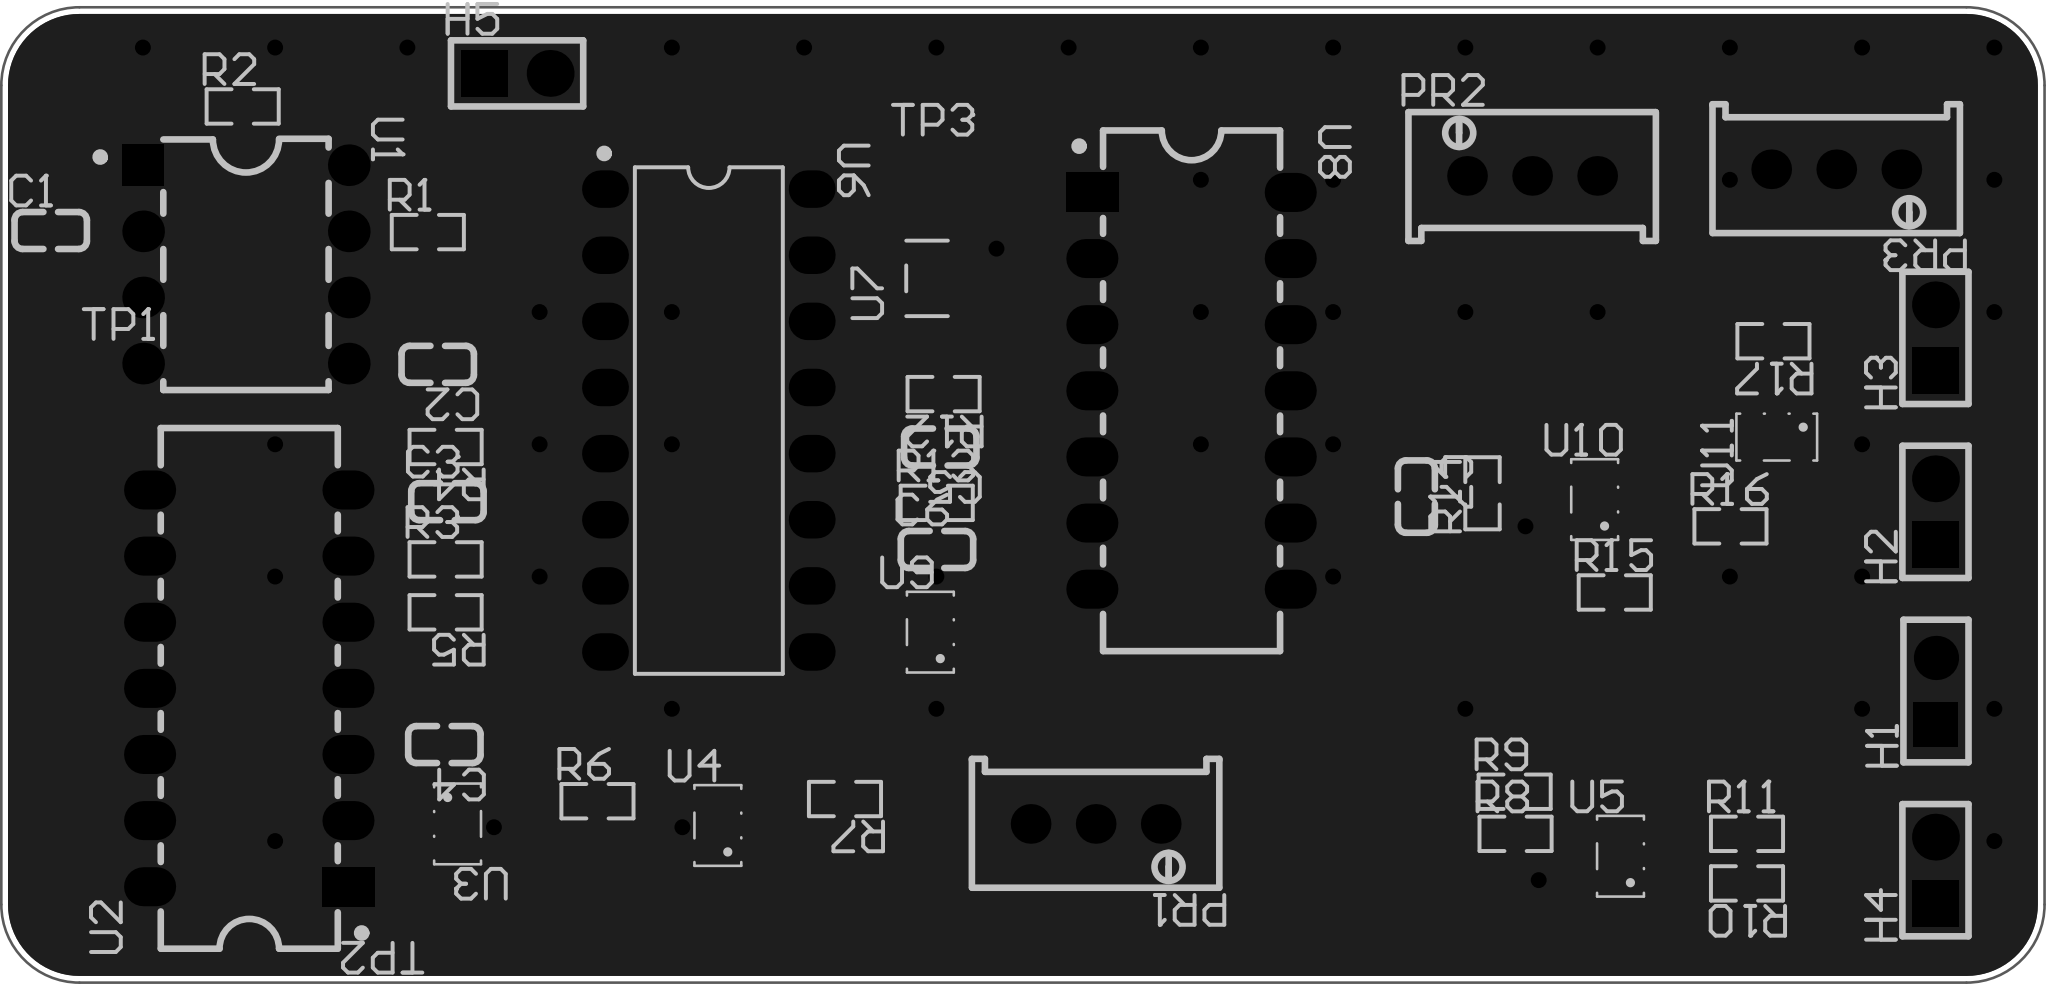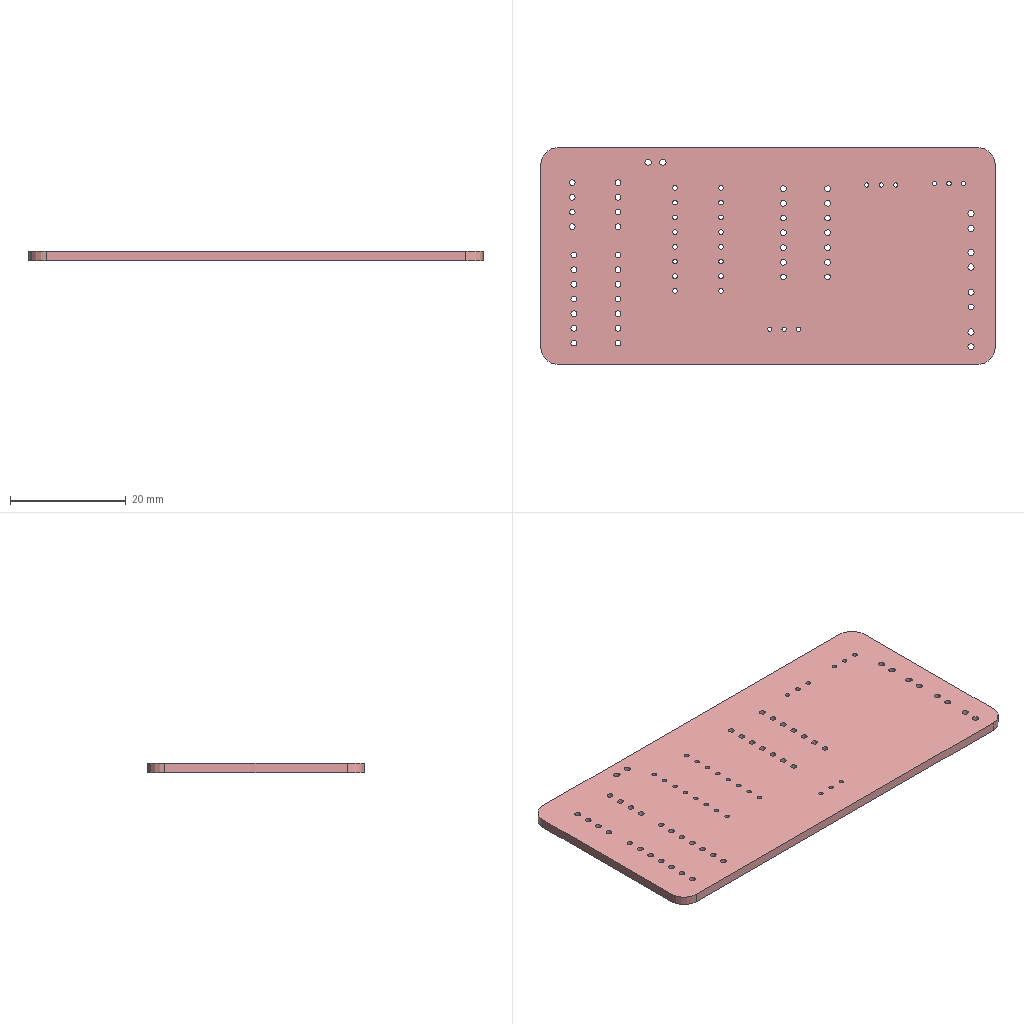Circuit board layout | Altium Designer | box 78.5 x 37.5 x 1.6 mm
Layer stack:
# Altium Designer layer stack of  (unit mm; dielectric type: 0 none, 1 core, 2 prepreg, 3 surface material)
index,name,kind,layer,copper_thickness_mm,dielectric_type,dielectric_thickness_mm,dielectric_material,dielectric_constant
0,Top Paste Mask Layer,other,,,,,,
1,Top Silkscreen Layer,other,,,,,,
2,Top Solder Mask Layer,dielectric,,,3,0.01,,3.3
3,Top Layer,copper,Top Layer,0.035,,,,
4,Dielectric1,dielectric,,,3,1.51,FR4,4.5
5,Bottom Layer,copper,Bottom Layer,0.035,,,,
6,Bottom Solder Mask Layer,dielectric,,,3,0.01,,3.3
7,Bottom Silkscreen Layer,other,,,,,,
8,Bottom Paste Mask Layer,other,,,,,,
# drill layer pairs: low layer,high layer
drill_pair,Top Layer,Bottom Layer
Part placement:
Designator,Comment,Layer,Footprint,Center-X(mm),Center-Y(mm),Rotation
C1,5nF,TopLayer,C0603,79.876,108.011,0
C2,0.22uF,TopLayer,C0603,94.742,102.87,180
C3,5.1nF,TopLayer,C0603,95.114,97.596,0
C4,1nF,TopLayer,C0603,94.996,88.265,180
C5,3300pF,TopLayer,C0603,114.046,99.695,180
C6,3300pF,TopLayer,C0603,113.919,95.758,0
C7,1nF,TopLayer,C0603,132.334,97.79,270
H1,,TopLayer,HDR-TH_2P-P2.54-V-F,152.293,90.321,90
H2,,TopLayer,HDR-TH_2P-P2.54-V-M-1,152.273,97.204,90
H3,,TopLayer,HDR-TH_2P-P2.54-V-M-1,152.273,103.886,90
H4,,TopLayer,HDR-TH_2P-P2.54-V-M-1,152.273,83.439,90
PR1,10kΩ,TopLayer,R_3296,120.015,85.217,180
PR2,10kΩ,TopLayer,R_3296,136.779,110.109,0
PR3,10kΩ,TopLayer,R_3296,148.463,110.363,180
R1,1.2K,TopLayer,R0603,94.361,107.95,0
R2,1.8K,TopLayer,R0603,87.249,112.776,0
R3,2K,TopLayer,R0603,95.044,95.377,0
R4,2K,TopLayer,R0603,95.044,99.695,180
R5,2.7K,TopLayer,R0603,95.044,93.345,180
R6,2K,TopLayer,R0603,100.877,86.089,0
R7,2K,TopLayer,R0603,110.385,86.173,180
R8,10K,TopLayer,R0603,136.144,84.836,0
R9,10K,TopLayer,R0603,136.109,86.453,0
R10,10K,TopLayer,R0603,145.034,82.931,180
R11,10K,TopLayer,R0603,145.034,84.836,0
R12,5.1K,TopLayer,R0603,114.173,101.727,180
R13,5.1K,TopLayer,R0603,113.909,97.549,0
R14,10K,TopLayer,R0603,134.874,97.917,90
R15,10K,TopLayer,R0603,139.954,94.107,0
R16,2K,TopLayer,R0603,144.399,96.647,0
R17,2K,TopLayer,R0603,146.05,103.759,180
TP1,,TopLayer,Test-Point-0.5mm,81.394,103.471,0
TP2,,TopLayer,Test-Point-0.5mm,93.901,81.026,180
TP3,,TopLayer,Test-Point-0.5mm,112.478,111.318,0
U1,NE555,TopLayer,PDIP-8_L9.6-W6.4-P2.54-LS7.9-BL-1,87.375,106.709,270
U2,DM7474N,TopLayer,PDIP-14_L19.5-W6.7-P2.54-LS7.9-BL,87.503,90.424,90
U3,OPAMP_3T_VIRTUAL,TopLayer,SOT-23-5_L3.0-W1.7-P0.95-LS2.8-BR,95.504,85.217,180
U4,OPAMP_3T_VIRTUAL,TopLayer,SOT-23-5_L3.0-W1.7-P0.95-LS2.8-BR,105.502,85.157,0
U5,OPAMP_3T_VIRTUAL,TopLayer,SOT-23-5_L3.0-W1.7-P0.95-LS2.8-BR,140.175,83.976,0
U6,74LS161N,TopLayer,PDIP-16_L19.3-W6.4-P2.54-LS7.94-BL,105.156,100.711,270
U7,HSN74LVC1G04DBVR,TopLayer,SOT-23-5_L2.9-W1.6-P0.95-LS2.9-BL,113.538,106.172,90
U8,DM7474N,TopLayer,PDIP-14_L19.5-W6.7-P2.54-LS7.9-BL,123.698,101.854,270
U9,OPAMP_3T_VIRTUAL,TopLayer,SOT-23-5_L3.0-W1.7-P0.95-LS2.8-BR,113.665,92.583,0
U10,OPAMP_3T_VIRTUAL,TopLayer,SOT-23-5_L3.0-W1.7-P0.95-LS2.8-BR,139.182,97.676,0
U11,OPAMP_3T_VIRTUAL,TopLayer,SOT-23-5_L3.0-W1.7-P0.95-LS2.8-BR,146.177,100.076,90
H5,,TopLayer,HDR-TH_2P-P2.54-V-M-1,97.79,114.046,0
Pad and via stacks:
# Altium Designer via and pad stacks of  (unit mm). Each distinct definition once, with the count of objects using it.
# via: kind,start_layer,end_layer,hole_mm,diameter_mm,mode(0 simple;1 top-mid-bottom;2 full stack),diameter_per_layer,count,example_net
# pad: kind,layer,hole_mm,hole_type(0 round;1 square;2 slot),plating,top_size,top_shape(1 round;2 rect;3 octagon;9 rounded rect),mid_size,bottom_size,mode,footprint,size_per_layer,count,example
pad,Top Layer,0,0,plated,0.8x0.9,2,0.8x0.9,0.8x0.9,0,C0603,,14,C1.2
pad,Top Layer,0,0,plated,0.8065x0.864,2,0.8065x0.864,0.8065x0.864,0,R0603,,34,R1.2
pad,Top Layer,0,0,plated,0.5x0.5,1,0.5x0.5,0.5x0.5,0,Test-Point-0.5mm,,3,TP1.1
pad,Top Layer,0,0,plated,1.1x0.6,2,1.1x0.6,1.1x0.6,0,SOT-23-5_L3.0-W1.7-P0.95-LS2.8-BR,,30,U3.5
pad,Top Layer,0,0,plated,0.6x1,2,0.6x1,0.6x1,0,SOT-23-5_L2.9-W1.6-P0.95-LS2.9-BL,,5,U7.5
pad,Multi-Layer,1,0,plated,1.7x1.7,2,1.7x1.7,1.7x1.7,0,HDR-TH_2P-P2.54-V-F,,1,H1.1
pad,Multi-Layer,1,0,plated,1.7x1.7,1,1.7x1.7,1.7x1.7,0,HDR-TH_2P-P2.54-V-F,,1,H1.2
pad,Multi-Layer,1.1,0,plated,1.8x1.8,1,1.8x1.8,1.8x1.8,0,HDR-TH_2P-P2.54-V-M-1,,4,H2.2
pad,Multi-Layer,1.1,0,plated,1.8x1.8,2,1.8x1.8,1.8x1.8,0,HDR-TH_2P-P2.54-V-M-1,,4,H2.1
pad,Multi-Layer,0.762,0,plated,1.524x1.524,1,1.524x1.524,1.524x1.524,0,R_3296,,9,PR1.2
pad,Multi-Layer,1,0,plated,1.6x1.6,1,1.6x1.6,1.6x1.6,0,PDIP-8_L9.6-W6.4-P2.54-LS7.9-BL-1,,7,U1.8
pad,Multi-Layer,1,0,plated,1.6x1.6,2,1.6x1.6,1.6x1.6,0,PDIP-8_L9.6-W6.4-P2.54-LS7.9-BL-1,,1,U1.1
pad,Multi-Layer,1,0,plated,2x1.5,1,2x1.5,2x1.5,0,PDIP-14_L19.5-W6.7-P2.54-LS7.9-BL,,26,U2.8
pad,Multi-Layer,1,0,plated,2x1.5,2,2x1.5,2x1.5,0,PDIP-14_L19.5-W6.7-P2.54-LS7.9-BL,,2,U2.1
pad,Multi-Layer,0.8,0,plated,1.44x1.8,1,1.44x1.8,1.44x1.8,0,PDIP-16_L19.3-W6.4-P2.54-LS7.94-BL,,16,U6.1
via,Top Layer,Bottom Layer,0.3048,0.6096,0,,4,VCC
via,Top Layer,Bottom Layer,0.3048,0.61,0,,45,GND
Copper pours:
name,layer,net,type(0 solid;1 hatched;2 none)
Top Layer-GND,Top Layer,GND,0
Bottom Layer-GND,Bottom Layer,GND,0